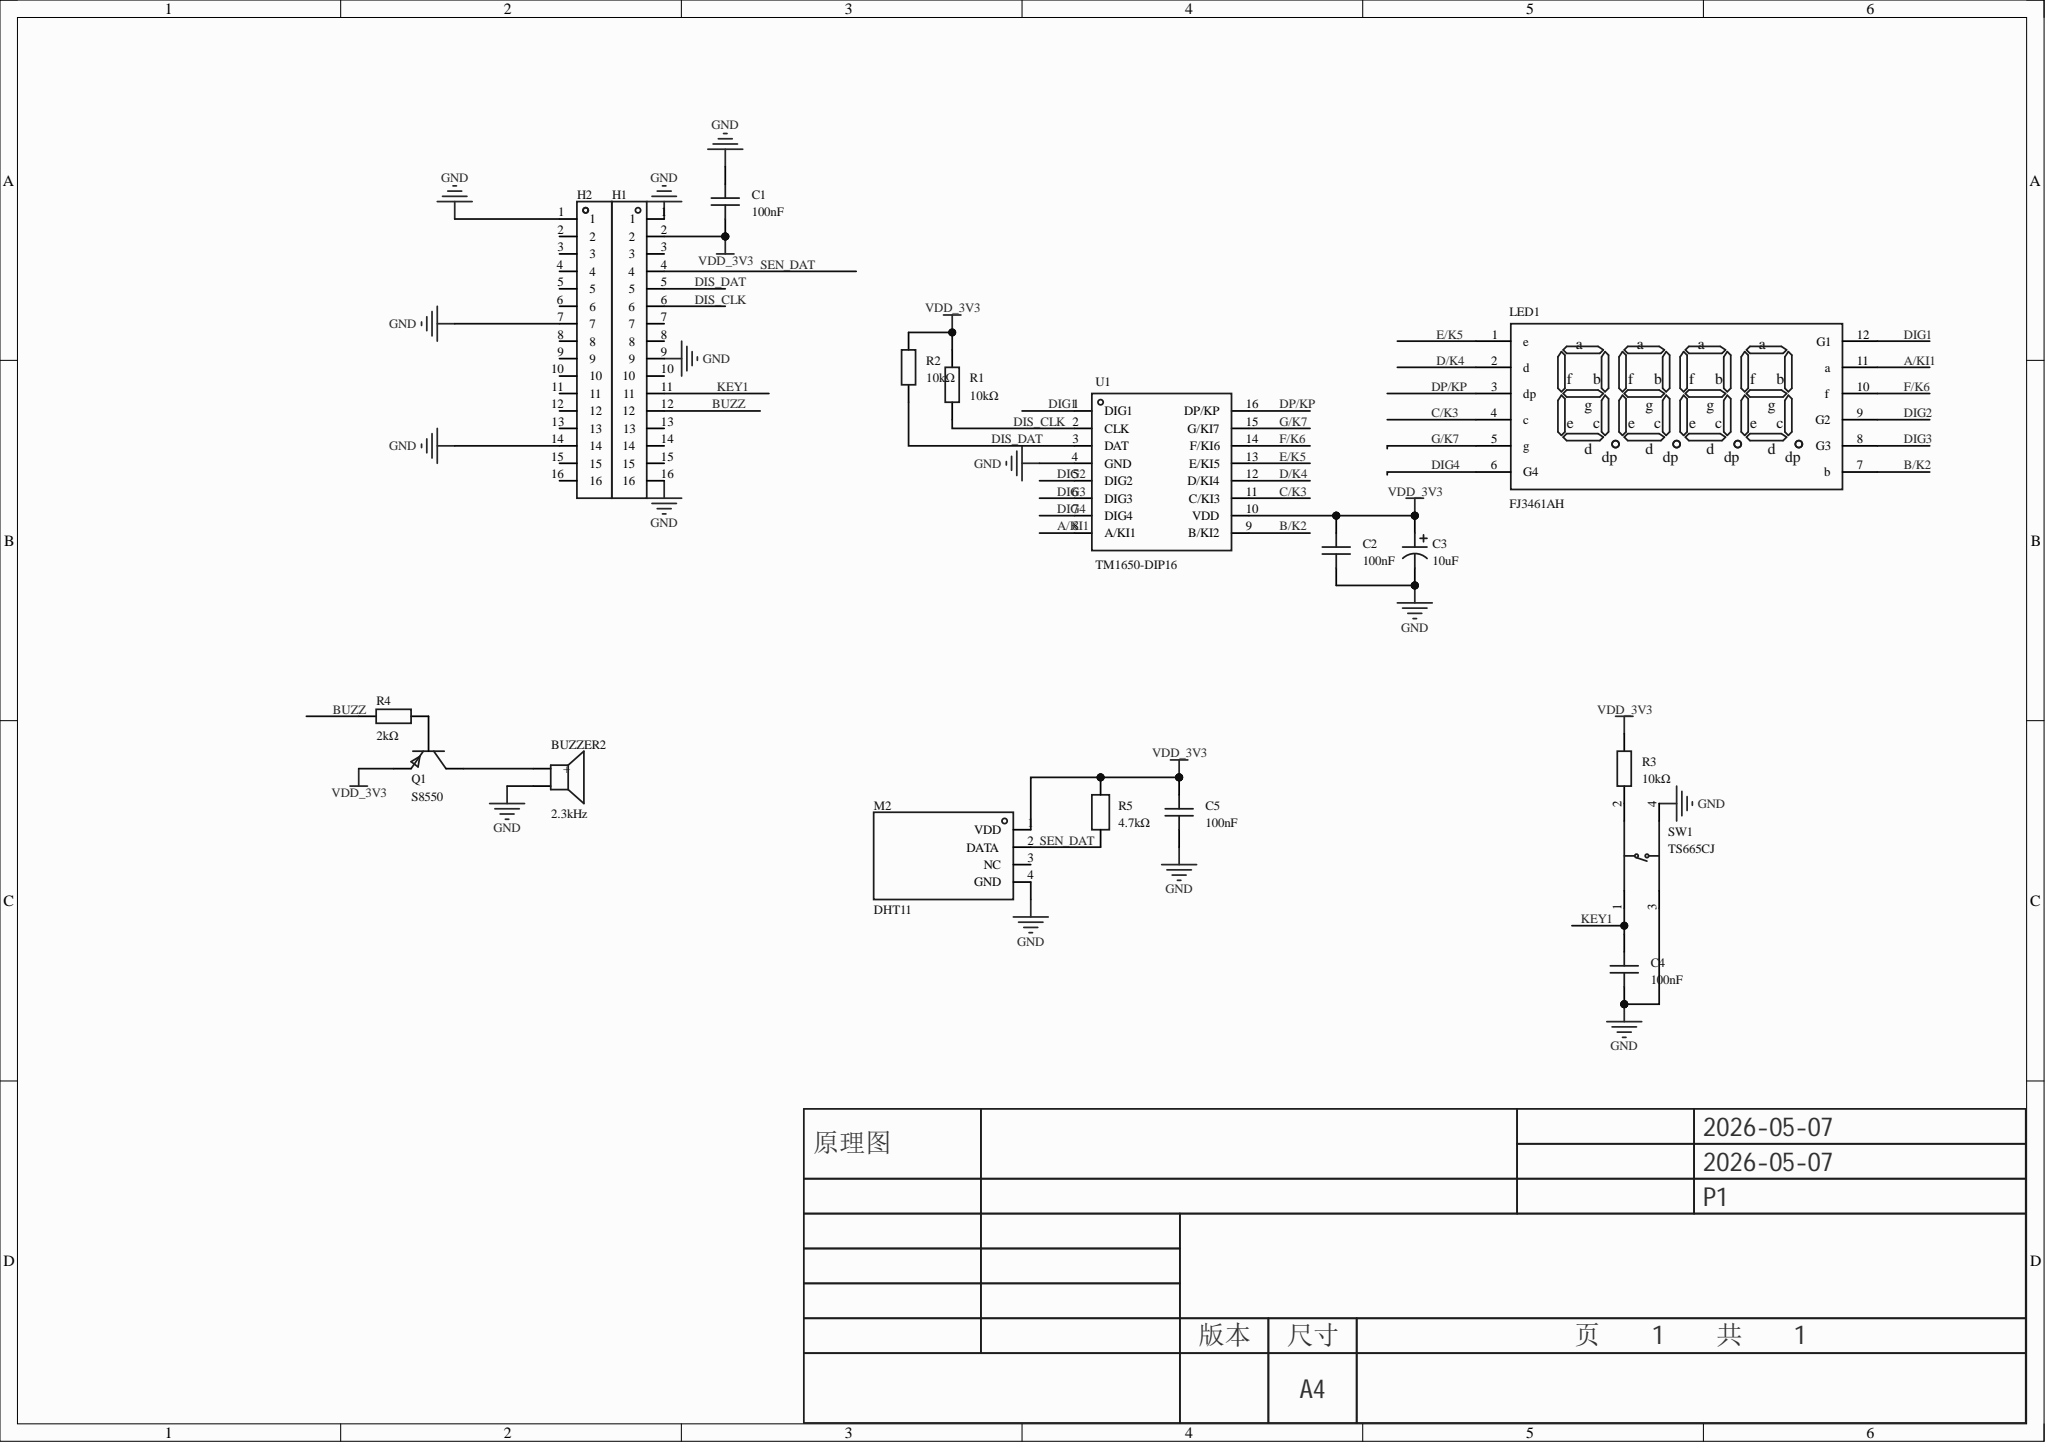Circuit board | Altium Designer | 18 parts | 22 nets
Bill of materials:
Comment,Description,Designator,Footprint,LibRef,Quantity
"2.3kHz","驱动方式:有源(内含驱动线路);构造类型:电磁式;额定电压:3V;频率:2.3kHz;声压(SPL):85dB;","BUZZER2","BUZ-TH_BD12.0-P7.60-D0.6-FD","TMB12A03","1"
"100nF","容值:100nF;精度:-20%~+80%;额定电压:50V;温度系数:Y5V;","C1, C2, C4, C5","CAP-TH_L5.8-W2.4-P2.54-D0.6","CC1H104ZA1PD3F5O3100","4"
"10uF","","C3","CAP-TH_BD5.0-P2.00-D0.8-FD","01EC1777","1"
"","","H1, H2","HDR-TH_16P-P2.54-V-F","HDR-F_2.54_1x16P","2"
"FJ3461AH","数码管位数:4位;字符尺寸(英寸):0.36;耗散功率(Pd):-;发光颜色:红色;LED极性:共阴极;","LED1","LED-SEG-TH_12P-L30.0-W14.0-P2.54-S10.16-BL","FJ3461AH","1"
"DHT11","温度范围:-20℃~+60℃;湿度范围:5%RH~95%RH;湿度精度:±5%RH;","M2","SENSOR-TH_DHT11","DHT11","1"
"S8550","晶体管类型:PNP;集电极电流(Ic):500mA;集射极击穿电压(Vceo):25V;耗散功率(Pd):625mW;直流电流增益(hFE):160@50mA,1V;","Q1","TO-92-3_L4.5-W3.5-P1.27-L","S8550_C2931493","1"
"10kΩ","","R1, R2, R3","R1206","1206W4J0103T5E","3"
"2kΩ","","R4","RES-TH_BD2.4-L6.3-P10.30-D0.6","MFR-25FBF52-2K","1"
"4.7kΩ","","R5","RES-TH_BD2.4-L6.3-P10.30-D0.6","MFR-25FBF52-4K7","1"
"TS665CJ","电路结构:单刀单掷;按钮形状:圆形按钮;作用力:2.5N;安装方式:直插;开关长度:6mm;开关宽度:6mm;开关高度:5mm;带支架:不带支架;触点电流:50mA;额定电压:12V;带灯:无;工作寿命:5万次;","SW1","SW-TH_4P-L6.0-W6.0-P4.50-LS6.5","TS665CJ","1"
"TM1650-DIP16","类型:-;工作电压(DC):3V~5.5V;开关频率:-;通道数:-;输出电压:-;输出电流:150mA;调光:-;拓扑结构:-;","U1","DIP-16_L19.3-W6.4-P2.54-LS8.0-BL","TM1650-DIP16","1"
Netlist (Protel format):
[
BUZZER2
BUZ-TH_BD12.0-P7.60-D0.6-FD
2.3kHz



]
[
C1
CAP-TH_L5.8-W2.4-P2.54-D0.6
100nF



]
[
C2
CAP-TH_L5.8-W2.4-P2.54-D0.6
100nF



]
[
C3
CAP-TH_BD5.0-P2.00-D0.8-FD
10uF



]
[
C4
CAP-TH_L5.8-W2.4-P2.54-D0.6
100nF



]
[
C5
CAP-TH_L5.8-W2.4-P2.54-D0.6
100nF



]
[
H1
HDR-TH_16P-P2.54-V-F




]
[
H2
HDR-TH_16P-P2.54-V-F




]
[
LED1
LED-SEG-TH_12P-L30.0-W14.0-P2.54-S10.16-BL
FJ3461AH



]
[
M2
SENSOR-TH_DHT11
DHT11



]
[
Q1
TO-92-3_L4.5-W3.5-P1.27-L
S8550



]
[
R1
R1206
10kΩ



]
[
R2
R1206
10kΩ



]
[
R3
R1206
10kΩ



]
[
R4
RES-TH_BD2.4-L6.3-P10.30-D0.6
2kΩ



]
[
R5
RES-TH_BD2.4-L6.3-P10.30-D0.6
4.7kΩ



]
[
SW1
SW-TH_4P-L6.0-W6.0-P4.50-LS6.5
TS665CJ



]
[
U1
DIP-16_L19.3-W6.4-P2.54-LS8.0-BL
TM1650-DIP16



]
(
VDD_3V3
C1-1
C2-2
C3-1
C5-2
H1-2
M2-1
Q1-1
R1-2
R2-2
R3-2
R5-2
U1-10
)
(
SEN_DAT
H1-4
M2-2
R5-1
)
(
NetR3_1
R3-1
SW1-2
)
(
NetQ1_2
Q1-2
R4-2
)
(
NetBUZZER2_1
BUZZER2-1
Q1-3
)
(
KEY1
C4-2
H1-11
SW1-1
)
(
GND
BUZZER2-2
C1-2
C2-1
C3-2
C4-1
C5-1
H1-1
H1-9
H1-16
H2-1
H2-7
H2-14
M2-4
SW1-3
SW1-4
U1-4
)
(
G/K7
LED1-5
U1-15
)
(
F/K6
LED1-10
U1-14
)
(
E/K5
LED1-1
U1-13
)
(
DP/KP
LED1-3
U1-16
)
(
DIS_DAT
H1-5
R2-1
U1-3
)
(
DIS_CLK
H1-6
R1-1
U1-2
)
(
DIG4
LED1-6
U1-7
)
(
DIG3
LED1-8
U1-6
)
(
DIG2
LED1-9
U1-5
)
(
DIG1
LED1-12
U1-1
)
(
D/K4
LED1-2
U1-12
)
(
C/K3
LED1-4
U1-11
)
(
BUZZ
H1-12
R4-1
)
(
B/K2
LED1-7
U1-9
)
(
A/KI1
LED1-11
U1-8
)